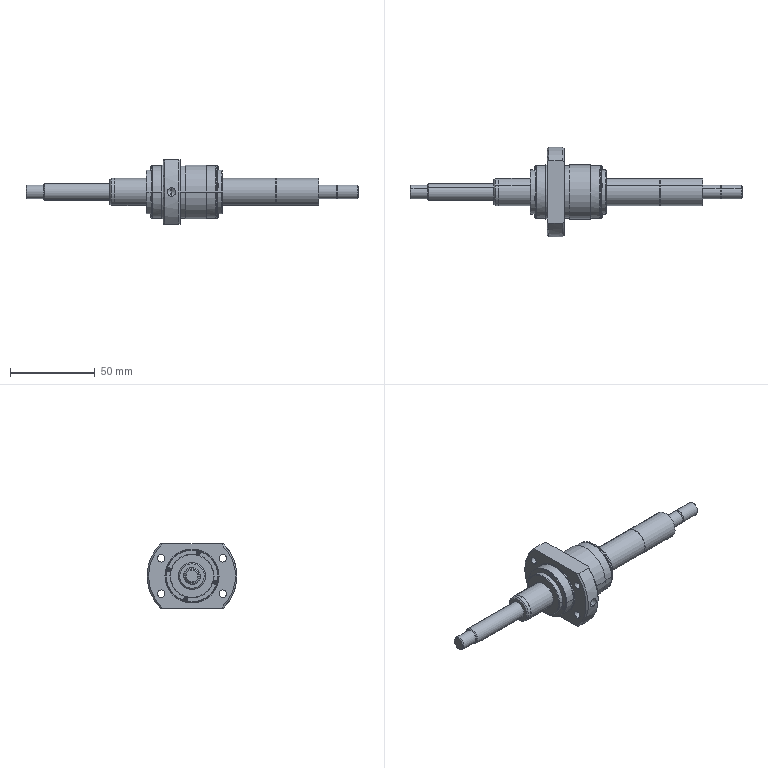Part | SolidWorks | features AEMSimFeature 1 | 2 solids | 229 faces | box 196 x 53 x 38 mm | volume 63498 mm3 | plane 136 | cylinder 69 | cone 20 | torus 4 | commonest cylinder face diameters 2.24 x16 31 x10 4.5 x8 16 x8 8 x6 12.8 x4